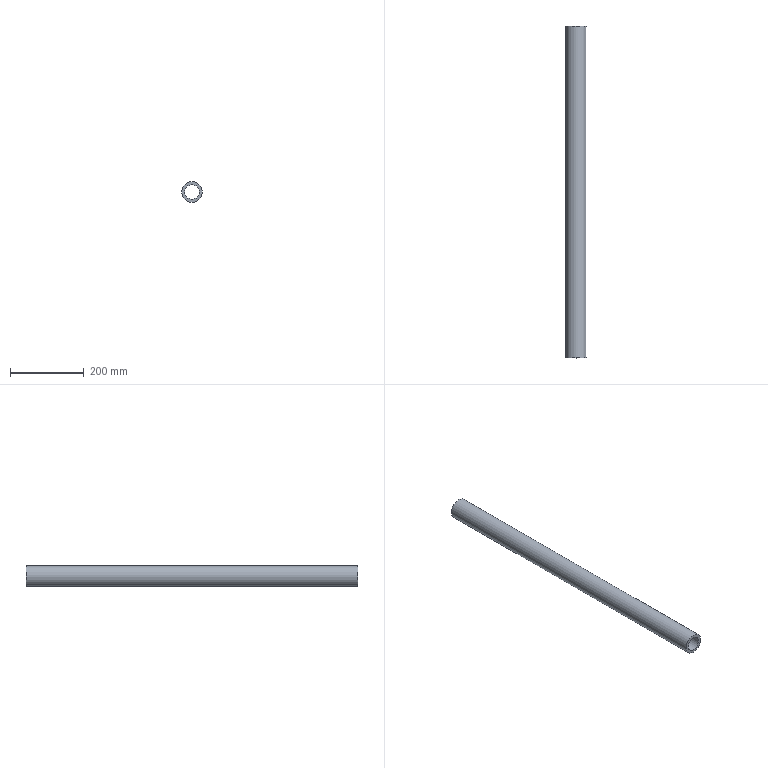Part | NX | features DATUM_CSYS 2, EXTRUDE 1, SKETCH 1 | 1 solid | 4 faces | box 56 x 902 x 56 mm | volume 1088147 mm3 | plane 2 | cylinder 2 | commonest cylinder face diameters 40 x1 56 x1
STEP:
#1=CARTESIAN_POINT('',(0.,451.,-28.));
#2=VERTEX_POINT('',#1);
#3=CARTESIAN_POINT('',(0.,451.,0.));
#4=DIRECTION('',(0.,-1.,0.));
#5=DIRECTION('',(0.,0.,-1.));
#6=AXIS2_PLACEMENT_3D('',#3,#4,#5);
#7=CIRCLE('',#6,28.);
#8=EDGE_CURVE('',#2,#2,#7,.T.);
#9=ORIENTED_EDGE('',*,*,#8,.F.);
#10=EDGE_LOOP('',(#9));
#11=FACE_BOUND('',#10,.T.);
#12=CARTESIAN_POINT('',(20.,451.,0.));
#13=VERTEX_POINT('',#12);
#14=CARTESIAN_POINT('',(0.,451.,0.));
#15=DIRECTION('',(0.,-1.,0.));
#16=DIRECTION('',(1.,0.,0.));
#17=AXIS2_PLACEMENT_3D('',#14,#15,#16);
#18=CIRCLE('',#17,20.);
#19=EDGE_CURVE('',#13,#13,#18,.T.);
#20=ORIENTED_EDGE('',*,*,#19,.T.);
#21=EDGE_LOOP('',(#20));
#22=FACE_BOUND('',#21,.T.);
#23=CARTESIAN_POINT('',(0.,451.,0.));
#24=DIRECTION('',(0.,1.,0.));
#25=DIRECTION('',(0.,0.,1.));
#26=AXIS2_PLACEMENT_3D('',#23,#24,#25);
#27=PLANE('',#26);
#28=ADVANCED_FACE('',(#11,#22),#27,.T.);
#29=CARTESIAN_POINT('',(0.,-451.,-28.));
#30=VERTEX_POINT('',#29);
#31=CARTESIAN_POINT('',(0.,-451.,0.));
#32=DIRECTION('',(0.,-1.,0.));
#33=DIRECTION('',(0.,0.,-1.));
#34=AXIS2_PLACEMENT_3D('',#31,#32,#33);
#35=CIRCLE('',#34,28.);
#36=EDGE_CURVE('',#30,#30,#35,.T.);
#37=ORIENTED_EDGE('',*,*,#36,.T.);
#38=EDGE_LOOP('',(#37));
#39=FACE_BOUND('',#38,.T.);
#40=CARTESIAN_POINT('',(20.,-451.,0.));
#41=VERTEX_POINT('',#40);
#42=CARTESIAN_POINT('',(0.,-451.,0.));
#43=DIRECTION('',(0.,-1.,0.));
#44=DIRECTION('',(1.,0.,0.));
#45=AXIS2_PLACEMENT_3D('',#42,#43,#44);
#46=CIRCLE('',#45,20.);
#47=EDGE_CURVE('',#41,#41,#46,.T.);
#48=ORIENTED_EDGE('',*,*,#47,.F.);
#49=EDGE_LOOP('',(#48));
#50=FACE_BOUND('',#49,.T.);
#51=CARTESIAN_POINT('',(0.,-451.,0.));
#52=DIRECTION('',(0.,1.,0.));
#53=DIRECTION('',(0.,0.,1.));
#54=AXIS2_PLACEMENT_3D('',#51,#52,#53);
#55=PLANE('',#54);
#56=ADVANCED_FACE('',(#39,#50),#55,.F.);
#57=ORIENTED_EDGE('',*,*,#8,.T.);
#58=EDGE_LOOP('',(#57));
#59=FACE_BOUND('',#58,.T.);
#60=ORIENTED_EDGE('',*,*,#36,.F.);
#61=EDGE_LOOP('',(#60));
#62=FACE_BOUND('',#61,.T.);
#63=CARTESIAN_POINT('',(0.,451.,0.));
#64=DIRECTION('',(0.,-1.,0.));
#65=DIRECTION('',(0.,0.,-1.));
#66=AXIS2_PLACEMENT_3D('',#63,#64,#65);
#67=CYLINDRICAL_SURFACE('',#66,28.);
#68=ADVANCED_FACE('',(#59,#62),#67,.T.);
#69=ORIENTED_EDGE('',*,*,#19,.F.);
#70=EDGE_LOOP('',(#69));
#71=FACE_BOUND('',#70,.T.);
#72=ORIENTED_EDGE('',*,*,#47,.T.);
#73=EDGE_LOOP('',(#72));
#74=FACE_BOUND('',#73,.T.);
#75=CARTESIAN_POINT('',(0.,451.,0.));
#76=DIRECTION('',(0.,-1.,0.));
#77=DIRECTION('',(0.,0.,-1.));
#78=AXIS2_PLACEMENT_3D('',#75,#76,#77);
#79=CYLINDRICAL_SURFACE('',#78,20.);
#80=ADVANCED_FACE('',(#71,#74),#79,.F.);
#81=CLOSED_SHELL('',(#28,#56,#68,#80));
#82=MANIFOLD_SOLID_BREP('',#81);
#83=(LENGTH_UNIT()NAMED_UNIT(*)SI_UNIT(.MILLI.,.METRE.));
#84=UNCERTAINTY_MEASURE_WITH_UNIT(LENGTH_MEASURE(0.00001),#83,'','');
#85=(NAMED_UNIT(*)PLANE_ANGLE_UNIT()SI_UNIT($,.RADIAN.));
#86=(NAMED_UNIT(*)SI_UNIT($,.STERADIAN.)SOLID_ANGLE_UNIT());
#87=(GEOMETRIC_REPRESENTATION_CONTEXT(3)GLOBAL_UNCERTAINTY_ASSIGNED_CONTEXT((#84))GLOBAL_UNIT_ASSIGNED_CONTEXT((#83,#85,#86))REPRESENTATION_CONTEXT('',''));
#88=ADVANCED_BREP_SHAPE_REPRESENTATION('',(#82),#87);